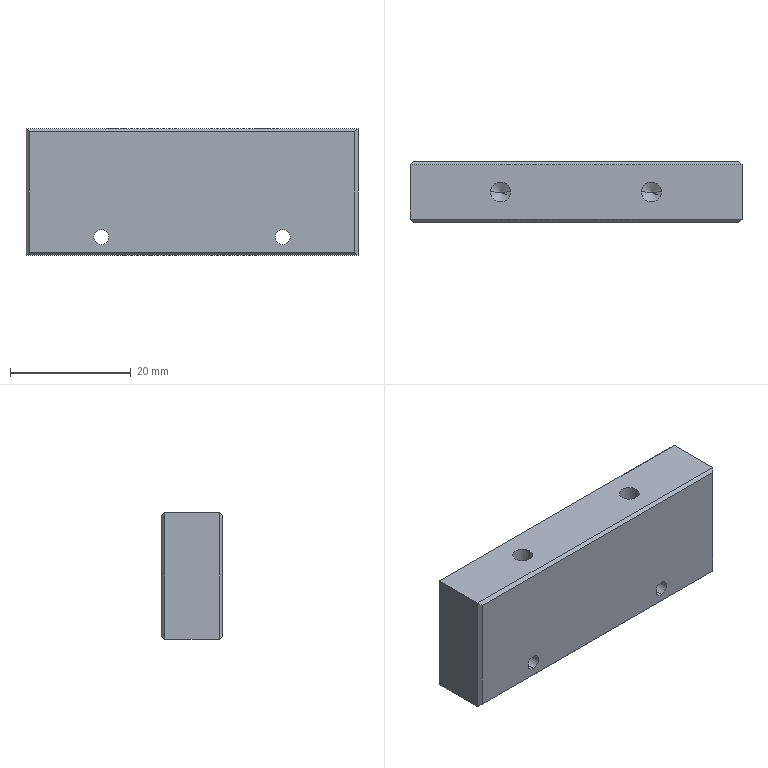Part | STEP file | GLSJ-10-16_default | 1 solid | 26 faces | box 55 x 10 x 21 mm | volume 11236 mm3 | plane 14 | cylinder 8 | cone 4 | commonest cylinder face diameters 2.5 x4 3.3 x4